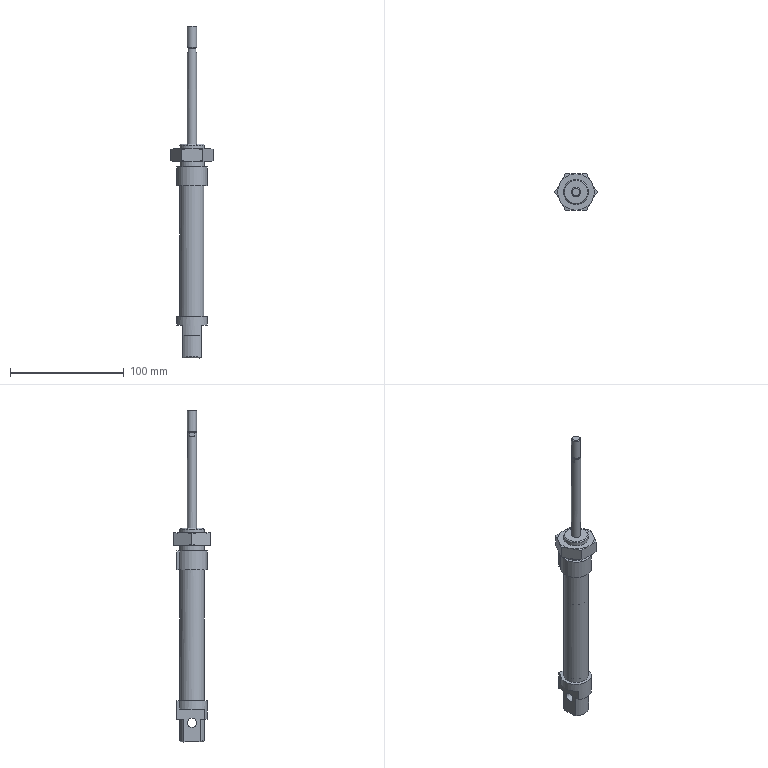Part | STEP file | 19211 DSNU-20-80-P-A | 3 solids | 71 faces | box 36.95 x 32 x 292 mm | volume 57538 mm3 | plane 35 | cone 21 | cylinder 15 | commonest cylinder face diameters 8 x4 22 x3 8.566 x2 20 x2 27 x2 20.16 x1